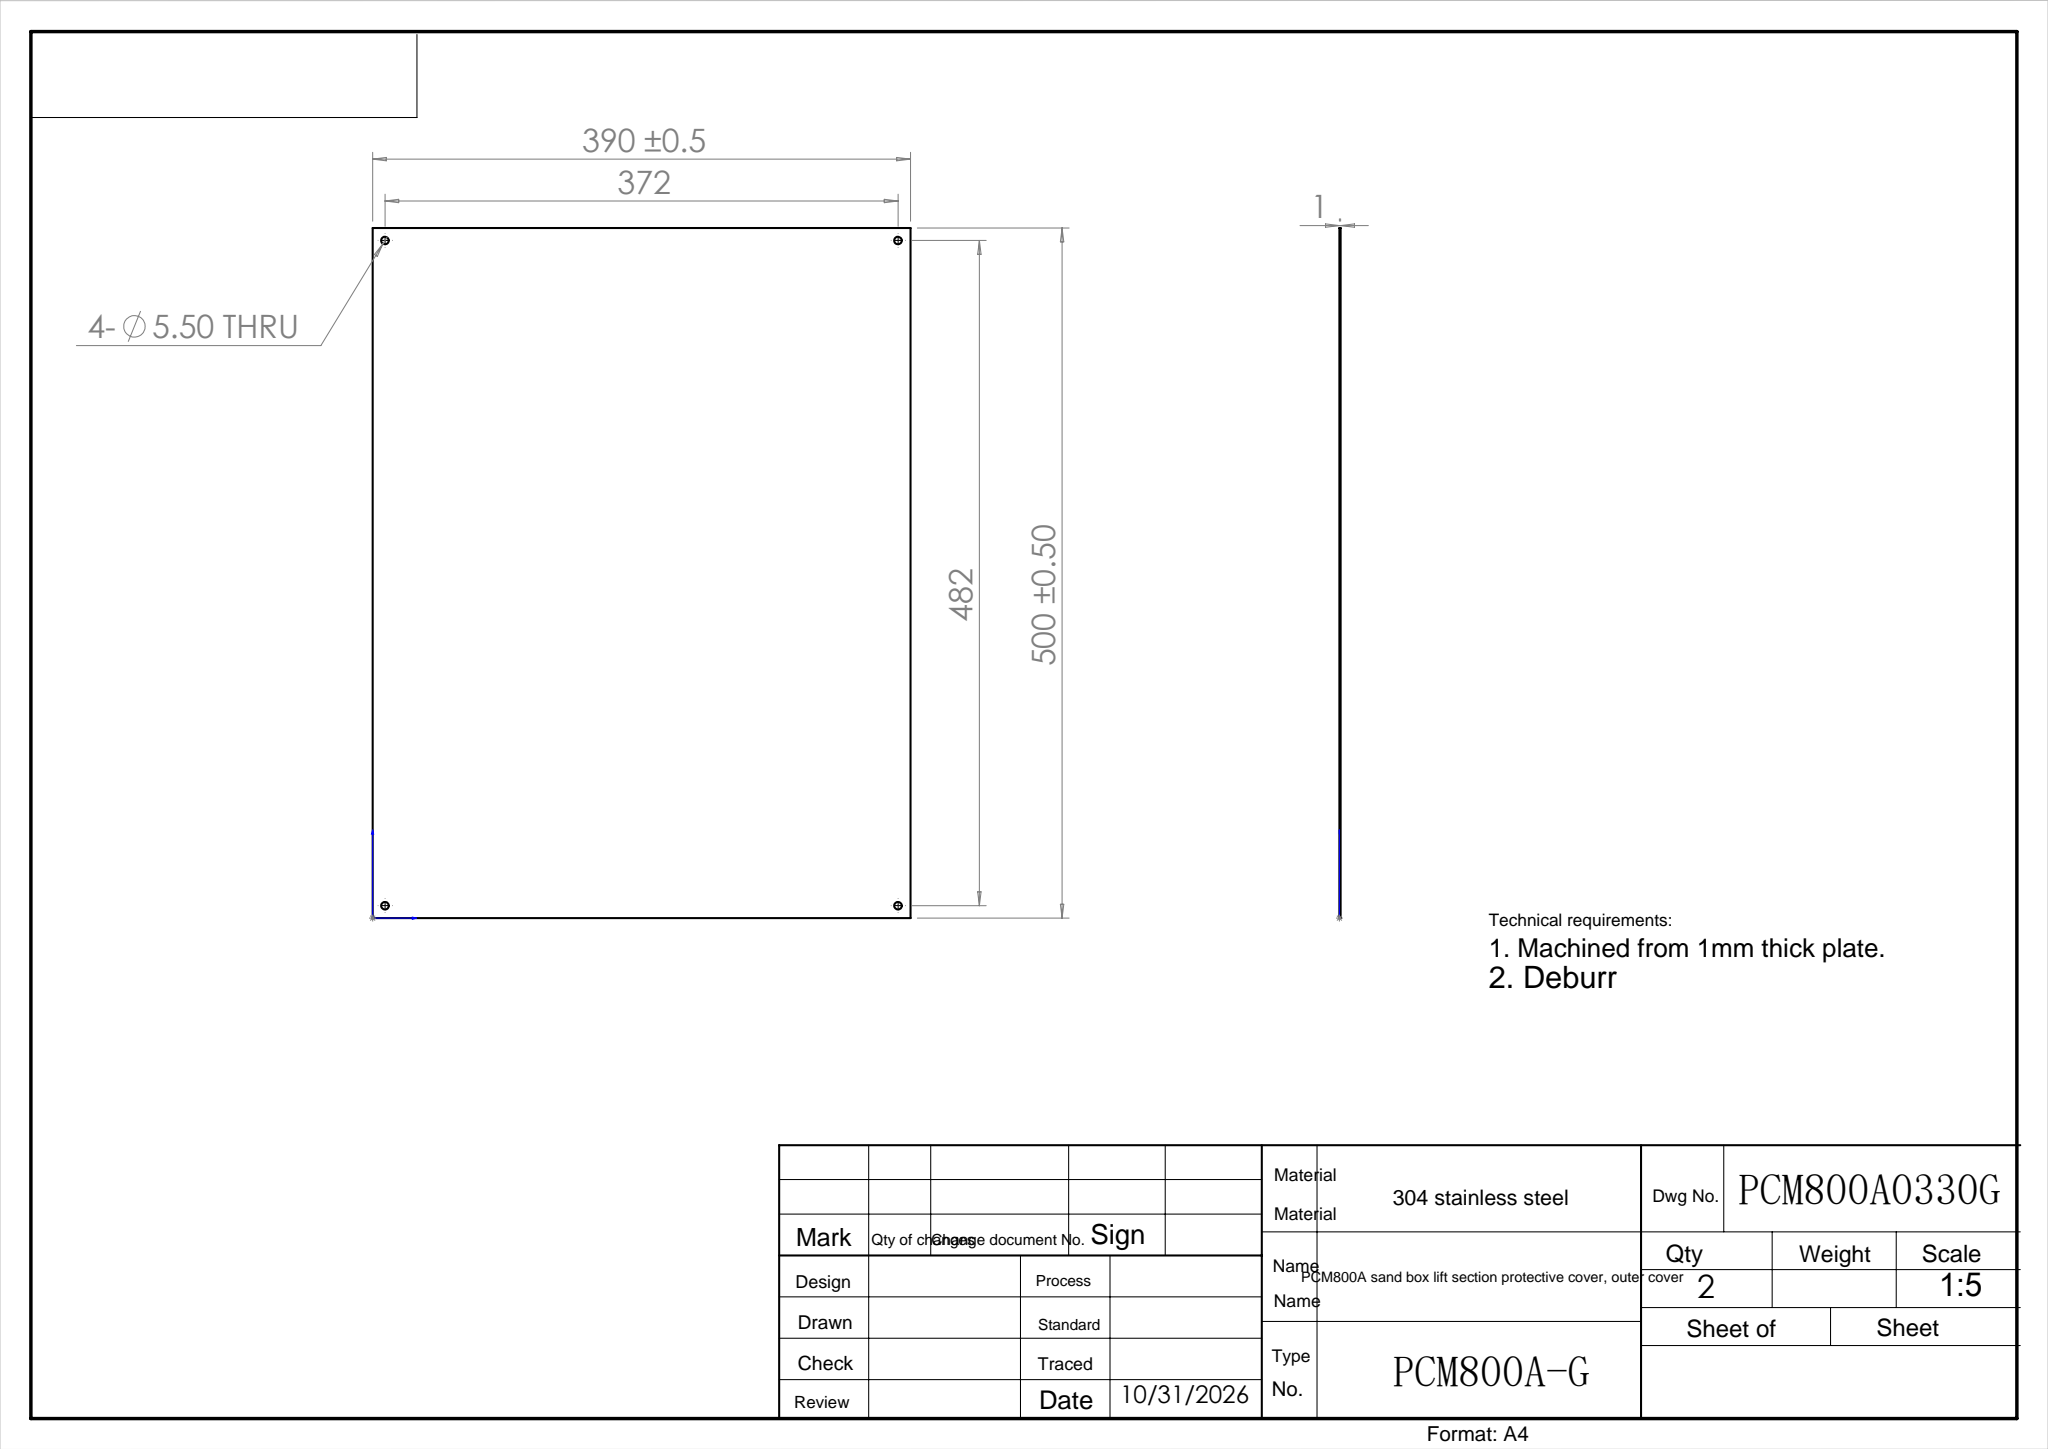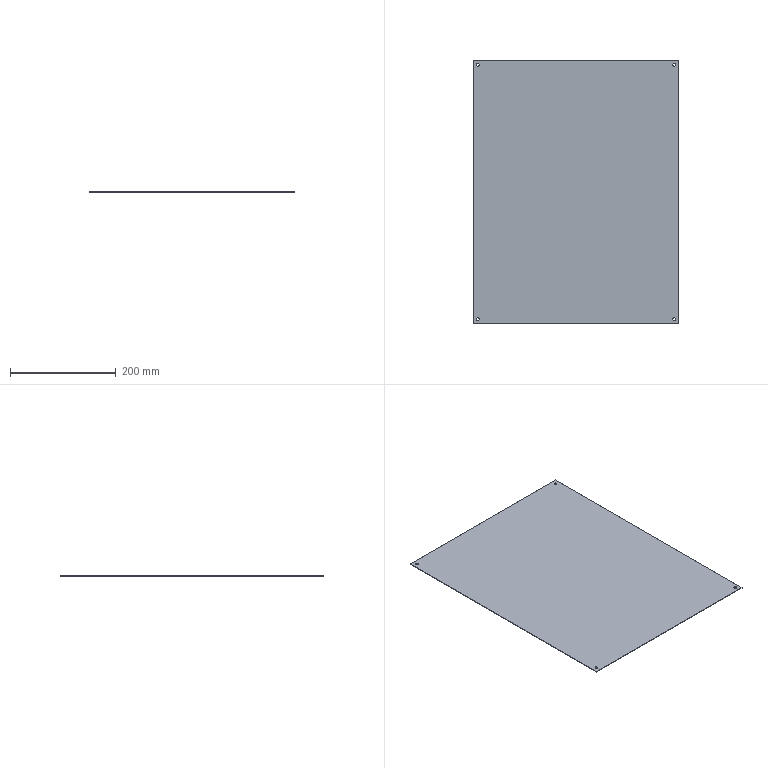Part | SolidWorks | features Extrusion 1, ICE 1 | 1 solid | 14 faces | box 390 x 500 x 1 mm | volume 194905 mm3 | cylinder 8 | plane 6 | commonest cylinder face diameters 5.5 x8
STEP:
#1=CARTESIAN_POINT('',(378.25,9.,0.));
#2=VERTEX_POINT('',#1);
#3=CARTESIAN_POINT('',(383.75,9.,0.));
#4=VERTEX_POINT('',#3);
#5=CARTESIAN_POINT('',(381.,9.,0.));
#6=DIRECTION('',(0.,0.,1.));
#7=DIRECTION('',(1.,0.,0.));
#8=AXIS2_PLACEMENT_3D('',#5,#6,#7);
#9=CIRCLE('',#8,2.75);
#10=EDGE_CURVE('',#2,#4,#9,.T.);
#11=ORIENTED_EDGE('',*,*,#10,.F.);
#12=CARTESIAN_POINT('',(378.25,9.,1.));
#13=VERTEX_POINT('',#12);
#14=CARTESIAN_POINT('',(378.25,9.,0.));
#15=DIRECTION('',(0.,0.,1.));
#16=VECTOR('',#15,1000.);
#17=LINE('',#14,#16);
#18=EDGE_CURVE('',#2,#13,#17,.T.);
#19=ORIENTED_EDGE('',*,*,#18,.T.);
#20=CARTESIAN_POINT('',(383.75,9.,1.));
#21=VERTEX_POINT('',#20);
#22=CARTESIAN_POINT('',(381.,9.,1.));
#23=DIRECTION('',(0.,0.,1.));
#24=DIRECTION('',(1.,0.,0.));
#25=AXIS2_PLACEMENT_3D('',#22,#23,#24);
#26=CIRCLE('',#25,2.75);
#27=EDGE_CURVE('',#13,#21,#26,.T.);
#28=ORIENTED_EDGE('',*,*,#27,.T.);
#29=CARTESIAN_POINT('',(383.75,9.,0.));
#30=DIRECTION('',(0.,0.,1.));
#31=VECTOR('',#30,1000.);
#32=LINE('',#29,#31);
#33=EDGE_CURVE('',#4,#21,#32,.T.);
#34=ORIENTED_EDGE('',*,*,#33,.F.);
#35=EDGE_LOOP('',(#11,#19,#28,#34));
#36=FACE_OUTER_BOUND('',#35,.T.);
#37=CARTESIAN_POINT('',(381.,9.,0.));
#38=DIRECTION('',(0.,0.,1.));
#39=DIRECTION('',(1.,0.,0.));
#40=AXIS2_PLACEMENT_3D('',#37,#38,#39);
#41=CYLINDRICAL_SURFACE('',#40,2.75);
#42=ADVANCED_FACE('',(#36),#41,.F.);
#43=CARTESIAN_POINT('',(6.25,9.,0.));
#44=VERTEX_POINT('',#43);
#45=CARTESIAN_POINT('',(11.75,9.,0.));
#46=VERTEX_POINT('',#45);
#47=CARTESIAN_POINT('',(9.,9.,0.));
#48=DIRECTION('',(0.,0.,1.));
#49=DIRECTION('',(1.,0.,0.));
#50=AXIS2_PLACEMENT_3D('',#47,#48,#49);
#51=CIRCLE('',#50,2.75);
#52=EDGE_CURVE('',#44,#46,#51,.T.);
#53=ORIENTED_EDGE('',*,*,#52,.F.);
#54=CARTESIAN_POINT('',(6.25,9.,1.));
#55=VERTEX_POINT('',#54);
#56=CARTESIAN_POINT('',(6.25,9.,0.));
#57=DIRECTION('',(0.,0.,1.));
#58=VECTOR('',#57,1000.);
#59=LINE('',#56,#58);
#60=EDGE_CURVE('',#44,#55,#59,.T.);
#61=ORIENTED_EDGE('',*,*,#60,.T.);
#62=CARTESIAN_POINT('',(11.75,9.,1.));
#63=VERTEX_POINT('',#62);
#64=CARTESIAN_POINT('',(9.,9.,1.));
#65=DIRECTION('',(0.,0.,1.));
#66=DIRECTION('',(1.,0.,0.));
#67=AXIS2_PLACEMENT_3D('',#64,#65,#66);
#68=CIRCLE('',#67,2.75);
#69=EDGE_CURVE('',#55,#63,#68,.T.);
#70=ORIENTED_EDGE('',*,*,#69,.T.);
#71=CARTESIAN_POINT('',(11.75,9.,0.));
#72=DIRECTION('',(0.,0.,1.));
#73=VECTOR('',#72,1000.);
#74=LINE('',#71,#73);
#75=EDGE_CURVE('',#46,#63,#74,.T.);
#76=ORIENTED_EDGE('',*,*,#75,.F.);
#77=EDGE_LOOP('',(#53,#61,#70,#76));
#78=FACE_OUTER_BOUND('',#77,.T.);
#79=CARTESIAN_POINT('',(9.,9.,0.));
#80=DIRECTION('',(0.,0.,1.));
#81=DIRECTION('',(1.,0.,0.));
#82=AXIS2_PLACEMENT_3D('',#79,#80,#81);
#83=CYLINDRICAL_SURFACE('',#82,2.75);
#84=ADVANCED_FACE('',(#78),#83,.F.);
#85=CARTESIAN_POINT('',(378.25,491.,0.));
#86=VERTEX_POINT('',#85);
#87=CARTESIAN_POINT('',(383.75,491.,0.));
#88=VERTEX_POINT('',#87);
#89=CARTESIAN_POINT('',(381.,491.,0.));
#90=DIRECTION('',(0.,0.,1.));
#91=DIRECTION('',(1.,0.,0.));
#92=AXIS2_PLACEMENT_3D('',#89,#90,#91);
#93=CIRCLE('',#92,2.75);
#94=EDGE_CURVE('',#86,#88,#93,.T.);
#95=ORIENTED_EDGE('',*,*,#94,.F.);
#96=CARTESIAN_POINT('',(378.25,491.,1.));
#97=VERTEX_POINT('',#96);
#98=CARTESIAN_POINT('',(378.25,491.,0.));
#99=DIRECTION('',(0.,0.,1.));
#100=VECTOR('',#99,1000.);
#101=LINE('',#98,#100);
#102=EDGE_CURVE('',#86,#97,#101,.T.);
#103=ORIENTED_EDGE('',*,*,#102,.T.);
#104=CARTESIAN_POINT('',(383.75,491.,1.));
#105=VERTEX_POINT('',#104);
#106=CARTESIAN_POINT('',(381.,491.,1.));
#107=DIRECTION('',(0.,0.,1.));
#108=DIRECTION('',(1.,0.,0.));
#109=AXIS2_PLACEMENT_3D('',#106,#107,#108);
#110=CIRCLE('',#109,2.75);
#111=EDGE_CURVE('',#97,#105,#110,.T.);
#112=ORIENTED_EDGE('',*,*,#111,.T.);
#113=CARTESIAN_POINT('',(383.75,491.,0.));
#114=DIRECTION('',(0.,0.,1.));
#115=VECTOR('',#114,1000.);
#116=LINE('',#113,#115);
#117=EDGE_CURVE('',#88,#105,#116,.T.);
#118=ORIENTED_EDGE('',*,*,#117,.F.);
#119=EDGE_LOOP('',(#95,#103,#112,#118));
#120=FACE_OUTER_BOUND('',#119,.T.);
#121=CARTESIAN_POINT('',(381.,491.,0.));
#122=DIRECTION('',(0.,0.,1.));
#123=DIRECTION('',(1.,0.,0.));
#124=AXIS2_PLACEMENT_3D('',#121,#122,#123);
#125=CYLINDRICAL_SURFACE('',#124,2.75);
#126=ADVANCED_FACE('',(#120),#125,.F.);
#127=CARTESIAN_POINT('',(6.25,491.,0.));
#128=VERTEX_POINT('',#127);
#129=CARTESIAN_POINT('',(11.75,491.,0.));
#130=VERTEX_POINT('',#129);
#131=CARTESIAN_POINT('',(9.,491.,0.));
#132=DIRECTION('',(0.,0.,1.));
#133=DIRECTION('',(1.,0.,0.));
#134=AXIS2_PLACEMENT_3D('',#131,#132,#133);
#135=CIRCLE('',#134,2.75);
#136=EDGE_CURVE('',#128,#130,#135,.T.);
#137=ORIENTED_EDGE('',*,*,#136,.F.);
#138=CARTESIAN_POINT('',(6.25,491.,1.));
#139=VERTEX_POINT('',#138);
#140=CARTESIAN_POINT('',(6.25,491.,0.));
#141=DIRECTION('',(0.,0.,1.));
#142=VECTOR('',#141,1000.);
#143=LINE('',#140,#142);
#144=EDGE_CURVE('',#128,#139,#143,.T.);
#145=ORIENTED_EDGE('',*,*,#144,.T.);
#146=CARTESIAN_POINT('',(11.75,491.,1.));
#147=VERTEX_POINT('',#146);
#148=CARTESIAN_POINT('',(9.,491.,1.));
#149=DIRECTION('',(0.,0.,1.));
#150=DIRECTION('',(1.,0.,0.));
#151=AXIS2_PLACEMENT_3D('',#148,#149,#150);
#152=CIRCLE('',#151,2.75);
#153=EDGE_CURVE('',#139,#147,#152,.T.);
#154=ORIENTED_EDGE('',*,*,#153,.T.);
#155=CARTESIAN_POINT('',(11.75,491.,0.));
#156=DIRECTION('',(0.,0.,1.));
#157=VECTOR('',#156,1000.);
#158=LINE('',#155,#157);
#159=EDGE_CURVE('',#130,#147,#158,.T.);
#160=ORIENTED_EDGE('',*,*,#159,.F.);
#161=EDGE_LOOP('',(#137,#145,#154,#160));
#162=FACE_OUTER_BOUND('',#161,.T.);
#163=CARTESIAN_POINT('',(9.,491.,0.));
#164=DIRECTION('',(0.,0.,1.));
#165=DIRECTION('',(1.,0.,0.));
#166=AXIS2_PLACEMENT_3D('',#163,#164,#165);
#167=CYLINDRICAL_SURFACE('',#166,2.75);
#168=ADVANCED_FACE('',(#162),#167,.F.);
#169=CARTESIAN_POINT('',(0.,500.,0.));
#170=VERTEX_POINT('',#169);
#171=CARTESIAN_POINT('',(0.,0.,0.));
#172=VERTEX_POINT('',#171);
#173=CARTESIAN_POINT('',(0.,0.,0.));
#174=DIRECTION('',(0.,-1.,0.));
#175=VECTOR('',#174,1000.);
#176=LINE('',#173,#175);
#177=EDGE_CURVE('',#170,#172,#176,.T.);
#178=ORIENTED_EDGE('',*,*,#177,.T.);
#179=CARTESIAN_POINT('',(0.,0.,1.));
#180=VERTEX_POINT('',#179);
#181=CARTESIAN_POINT('',(0.,0.,1.));
#182=DIRECTION('',(0.,0.,-1.));
#183=VECTOR('',#182,1000.);
#184=LINE('',#181,#183);
#185=EDGE_CURVE('',#180,#172,#184,.T.);
#186=ORIENTED_EDGE('',*,*,#185,.F.);
#187=CARTESIAN_POINT('',(0.,500.,1.));
#188=VERTEX_POINT('',#187);
#189=CARTESIAN_POINT('',(0.,0.,1.));
#190=DIRECTION('',(0.,-1.,0.));
#191=VECTOR('',#190,1000.);
#192=LINE('',#189,#191);
#193=EDGE_CURVE('',#188,#180,#192,.T.);
#194=ORIENTED_EDGE('',*,*,#193,.F.);
#195=CARTESIAN_POINT('',(0.,500.,1.));
#196=DIRECTION('',(0.,0.,-1.));
#197=VECTOR('',#196,1000.);
#198=LINE('',#195,#197);
#199=EDGE_CURVE('',#188,#170,#198,.T.);
#200=ORIENTED_EDGE('',*,*,#199,.T.);
#201=EDGE_LOOP('',(#178,#186,#194,#200));
#202=FACE_OUTER_BOUND('',#201,.T.);
#203=CARTESIAN_POINT('',(0.,0.,1.));
#204=DIRECTION('',(1.,0.,0.));
#205=DIRECTION('',(0.,0.,-1.));
#206=AXIS2_PLACEMENT_3D('',#203,#204,#205);
#207=PLANE('',#206);
#208=ADVANCED_FACE('',(#202),#207,.F.);
#209=CARTESIAN_POINT('',(390.,0.,0.));
#210=VERTEX_POINT('',#209);
#211=CARTESIAN_POINT('',(0.,0.,0.));
#212=DIRECTION('',(1.,0.,0.));
#213=VECTOR('',#212,1000.);
#214=LINE('',#211,#213);
#215=EDGE_CURVE('',#172,#210,#214,.T.);
#216=ORIENTED_EDGE('',*,*,#215,.T.);
#217=CARTESIAN_POINT('',(390.,0.,1.));
#218=VERTEX_POINT('',#217);
#219=CARTESIAN_POINT('',(390.,0.,1.));
#220=DIRECTION('',(0.,0.,-1.));
#221=VECTOR('',#220,1000.);
#222=LINE('',#219,#221);
#223=EDGE_CURVE('',#218,#210,#222,.T.);
#224=ORIENTED_EDGE('',*,*,#223,.F.);
#225=CARTESIAN_POINT('',(0.,0.,1.));
#226=DIRECTION('',(1.,0.,0.));
#227=VECTOR('',#226,1000.);
#228=LINE('',#225,#227);
#229=EDGE_CURVE('',#180,#218,#228,.T.);
#230=ORIENTED_EDGE('',*,*,#229,.F.);
#231=ORIENTED_EDGE('',*,*,#185,.T.);
#232=EDGE_LOOP('',(#216,#224,#230,#231));
#233=FACE_OUTER_BOUND('',#232,.T.);
#234=CARTESIAN_POINT('',(0.,0.,1.));
#235=DIRECTION('',(0.,1.,0.));
#236=DIRECTION('',(0.,0.,1.));
#237=AXIS2_PLACEMENT_3D('',#234,#235,#236);
#238=PLANE('',#237);
#239=ADVANCED_FACE('',(#233),#238,.F.);
#240=CARTESIAN_POINT('',(390.,500.,0.));
#241=VERTEX_POINT('',#240);
#242=CARTESIAN_POINT('',(390.,0.,0.));
#243=DIRECTION('',(0.,1.,0.));
#244=VECTOR('',#243,1000.);
#245=LINE('',#242,#244);
#246=EDGE_CURVE('',#210,#241,#245,.T.);
#247=ORIENTED_EDGE('',*,*,#246,.T.);
#248=CARTESIAN_POINT('',(390.,500.,1.));
#249=VERTEX_POINT('',#248);
#250=CARTESIAN_POINT('',(390.,500.,1.));
#251=DIRECTION('',(0.,0.,-1.));
#252=VECTOR('',#251,1000.);
#253=LINE('',#250,#252);
#254=EDGE_CURVE('',#249,#241,#253,.T.);
#255=ORIENTED_EDGE('',*,*,#254,.F.);
#256=CARTESIAN_POINT('',(390.,0.,1.));
#257=DIRECTION('',(0.,1.,0.));
#258=VECTOR('',#257,1000.);
#259=LINE('',#256,#258);
#260=EDGE_CURVE('',#218,#249,#259,.T.);
#261=ORIENTED_EDGE('',*,*,#260,.F.);
#262=ORIENTED_EDGE('',*,*,#223,.T.);
#263=EDGE_LOOP('',(#247,#255,#261,#262));
#264=FACE_OUTER_BOUND('',#263,.T.);
#265=CARTESIAN_POINT('',(390.,0.,1.));
#266=DIRECTION('',(-1.,0.,0.));
#267=DIRECTION('',(0.,0.,1.));
#268=AXIS2_PLACEMENT_3D('',#265,#266,#267);
#269=PLANE('',#268);
#270=ADVANCED_FACE('',(#264),#269,.F.);
#271=CARTESIAN_POINT('',(0.,500.,0.));
#272=DIRECTION('',(-1.,0.,0.));
#273=VECTOR('',#272,1000.);
#274=LINE('',#271,#273);
#275=EDGE_CURVE('',#241,#170,#274,.T.);
#276=ORIENTED_EDGE('',*,*,#275,.T.);
#277=ORIENTED_EDGE('',*,*,#199,.F.);
#278=CARTESIAN_POINT('',(0.,500.,1.));
#279=DIRECTION('',(-1.,0.,0.));
#280=VECTOR('',#279,1000.);
#281=LINE('',#278,#280);
#282=EDGE_CURVE('',#249,#188,#281,.T.);
#283=ORIENTED_EDGE('',*,*,#282,.F.);
#284=ORIENTED_EDGE('',*,*,#254,.T.);
#285=EDGE_LOOP('',(#276,#277,#283,#284));
#286=FACE_OUTER_BOUND('',#285,.T.);
#287=CARTESIAN_POINT('',(0.,500.,1.));
#288=DIRECTION('',(0.,-1.,0.));
#289=DIRECTION('',(0.,0.,-1.));
#290=AXIS2_PLACEMENT_3D('',#287,#288,#289);
#291=PLANE('',#290);
#292=ADVANCED_FACE('',(#286),#291,.F.);
#293=CARTESIAN_POINT('',(381.,9.,1.));
#294=DIRECTION('',(0.,0.,1.));
#295=DIRECTION('',(1.,0.,0.));
#296=AXIS2_PLACEMENT_3D('',#293,#294,#295);
#297=CIRCLE('',#296,2.75);
#298=EDGE_CURVE('',#21,#13,#297,.T.);
#299=ORIENTED_EDGE('',*,*,#298,.F.);
#300=ORIENTED_EDGE('',*,*,#27,.F.);
#301=EDGE_LOOP('',(#299,#300));
#302=FACE_BOUND('',#301,.T.);
#303=CARTESIAN_POINT('',(9.,9.,1.));
#304=DIRECTION('',(0.,0.,1.));
#305=DIRECTION('',(1.,0.,0.));
#306=AXIS2_PLACEMENT_3D('',#303,#304,#305);
#307=CIRCLE('',#306,2.75);
#308=EDGE_CURVE('',#63,#55,#307,.T.);
#309=ORIENTED_EDGE('',*,*,#308,.F.);
#310=ORIENTED_EDGE('',*,*,#69,.F.);
#311=EDGE_LOOP('',(#309,#310));
#312=FACE_BOUND('',#311,.T.);
#313=CARTESIAN_POINT('',(381.,491.,1.));
#314=DIRECTION('',(0.,0.,1.));
#315=DIRECTION('',(1.,0.,0.));
#316=AXIS2_PLACEMENT_3D('',#313,#314,#315);
#317=CIRCLE('',#316,2.75);
#318=EDGE_CURVE('',#105,#97,#317,.T.);
#319=ORIENTED_EDGE('',*,*,#318,.F.);
#320=ORIENTED_EDGE('',*,*,#111,.F.);
#321=EDGE_LOOP('',(#319,#320));
#322=FACE_BOUND('',#321,.T.);
#323=CARTESIAN_POINT('',(9.,491.,1.));
#324=DIRECTION('',(0.,0.,1.));
#325=DIRECTION('',(1.,0.,0.));
#326=AXIS2_PLACEMENT_3D('',#323,#324,#325);
#327=CIRCLE('',#326,2.75);
#328=EDGE_CURVE('',#147,#139,#327,.T.);
#329=ORIENTED_EDGE('',*,*,#328,.F.);
#330=ORIENTED_EDGE('',*,*,#153,.F.);
#331=EDGE_LOOP('',(#329,#330));
#332=FACE_BOUND('',#331,.T.);
#333=ORIENTED_EDGE('',*,*,#193,.T.);
#334=ORIENTED_EDGE('',*,*,#229,.T.);
#335=ORIENTED_EDGE('',*,*,#260,.T.);
#336=ORIENTED_EDGE('',*,*,#282,.T.);
#337=EDGE_LOOP('',(#333,#334,#335,#336));
#338=FACE_OUTER_BOUND('',#337,.T.);
#339=CARTESIAN_POINT('',(0.,500.,1.));
#340=DIRECTION('',(0.,0.,-1.));
#341=DIRECTION('',(-1.,0.,0.));
#342=AXIS2_PLACEMENT_3D('',#339,#340,#341);
#343=PLANE('',#342);
#344=ADVANCED_FACE('',(#302,#312,#322,#332,#338),#343,.F.);
#345=CARTESIAN_POINT('',(381.,9.,0.));
#346=DIRECTION('',(0.,0.,1.));
#347=DIRECTION('',(1.,0.,0.));
#348=AXIS2_PLACEMENT_3D('',#345,#346,#347);
#349=CIRCLE('',#348,2.75);
#350=EDGE_CURVE('',#4,#2,#349,.T.);
#351=ORIENTED_EDGE('',*,*,#350,.T.);
#352=ORIENTED_EDGE('',*,*,#10,.T.);
#353=EDGE_LOOP('',(#351,#352));
#354=FACE_BOUND('',#353,.T.);
#355=CARTESIAN_POINT('',(9.,9.,0.));
#356=DIRECTION('',(0.,0.,1.));
#357=DIRECTION('',(1.,0.,0.));
#358=AXIS2_PLACEMENT_3D('',#355,#356,#357);
#359=CIRCLE('',#358,2.75);
#360=EDGE_CURVE('',#46,#44,#359,.T.);
#361=ORIENTED_EDGE('',*,*,#360,.T.);
#362=ORIENTED_EDGE('',*,*,#52,.T.);
#363=EDGE_LOOP('',(#361,#362));
#364=FACE_BOUND('',#363,.T.);
#365=CARTESIAN_POINT('',(381.,491.,0.));
#366=DIRECTION('',(0.,0.,1.));
#367=DIRECTION('',(1.,0.,0.));
#368=AXIS2_PLACEMENT_3D('',#365,#366,#367);
#369=CIRCLE('',#368,2.75);
#370=EDGE_CURVE('',#88,#86,#369,.T.);
#371=ORIENTED_EDGE('',*,*,#370,.T.);
#372=ORIENTED_EDGE('',*,*,#94,.T.);
#373=EDGE_LOOP('',(#371,#372));
#374=FACE_BOUND('',#373,.T.);
#375=CARTESIAN_POINT('',(9.,491.,0.));
#376=DIRECTION('',(0.,0.,1.));
#377=DIRECTION('',(1.,0.,0.));
#378=AXIS2_PLACEMENT_3D('',#375,#376,#377);
#379=CIRCLE('',#378,2.75);
#380=EDGE_CURVE('',#130,#128,#379,.T.);
#381=ORIENTED_EDGE('',*,*,#380,.T.);
#382=ORIENTED_EDGE('',*,*,#136,.T.);
#383=EDGE_LOOP('',(#381,#382));
#384=FACE_BOUND('',#383,.T.);
#385=ORIENTED_EDGE('',*,*,#177,.F.);
#386=ORIENTED_EDGE('',*,*,#275,.F.);
#387=ORIENTED_EDGE('',*,*,#246,.F.);
#388=ORIENTED_EDGE('',*,*,#215,.F.);
#389=EDGE_LOOP('',(#385,#386,#387,#388));
#390=FACE_OUTER_BOUND('',#389,.T.);
#391=CARTESIAN_POINT('',(0.,500.,0.));
#392=DIRECTION('',(0.,0.,-1.));
#393=DIRECTION('',(-1.,0.,0.));
#394=AXIS2_PLACEMENT_3D('',#391,#392,#393);
#395=PLANE('',#394);
#396=ADVANCED_FACE('',(#354,#364,#374,#384,#390),#395,.T.);
#397=ORIENTED_EDGE('',*,*,#144,.F.);
#398=ORIENTED_EDGE('',*,*,#380,.F.);
#399=ORIENTED_EDGE('',*,*,#159,.T.);
#400=ORIENTED_EDGE('',*,*,#328,.T.);
#401=EDGE_LOOP('',(#397,#398,#399,#400));
#402=FACE_OUTER_BOUND('',#401,.T.);
#403=CARTESIAN_POINT('',(9.,491.,0.));
#404=DIRECTION('',(0.,0.,1.));
#405=DIRECTION('',(1.,0.,0.));
#406=AXIS2_PLACEMENT_3D('',#403,#404,#405);
#407=CYLINDRICAL_SURFACE('',#406,2.75);
#408=ADVANCED_FACE('',(#402),#407,.F.);
#409=ORIENTED_EDGE('',*,*,#102,.F.);
#410=ORIENTED_EDGE('',*,*,#370,.F.);
#411=ORIENTED_EDGE('',*,*,#117,.T.);
#412=ORIENTED_EDGE('',*,*,#318,.T.);
#413=EDGE_LOOP('',(#409,#410,#411,#412));
#414=FACE_OUTER_BOUND('',#413,.T.);
#415=CARTESIAN_POINT('',(381.,491.,0.));
#416=DIRECTION('',(0.,0.,1.));
#417=DIRECTION('',(1.,0.,0.));
#418=AXIS2_PLACEMENT_3D('',#415,#416,#417);
#419=CYLINDRICAL_SURFACE('',#418,2.75);
#420=ADVANCED_FACE('',(#414),#419,.F.);
#421=ORIENTED_EDGE('',*,*,#60,.F.);
#422=ORIENTED_EDGE('',*,*,#360,.F.);
#423=ORIENTED_EDGE('',*,*,#75,.T.);
#424=ORIENTED_EDGE('',*,*,#308,.T.);
#425=EDGE_LOOP('',(#421,#422,#423,#424));
#426=FACE_OUTER_BOUND('',#425,.T.);
#427=CARTESIAN_POINT('',(9.,9.,0.));
#428=DIRECTION('',(0.,0.,1.));
#429=DIRECTION('',(1.,0.,0.));
#430=AXIS2_PLACEMENT_3D('',#427,#428,#429);
#431=CYLINDRICAL_SURFACE('',#430,2.75);
#432=ADVANCED_FACE('',(#426),#431,.F.);
#433=ORIENTED_EDGE('',*,*,#18,.F.);
#434=ORIENTED_EDGE('',*,*,#350,.F.);
#435=ORIENTED_EDGE('',*,*,#33,.T.);
#436=ORIENTED_EDGE('',*,*,#298,.T.);
#437=EDGE_LOOP('',(#433,#434,#435,#436));
#438=FACE_OUTER_BOUND('',#437,.T.);
#439=CARTESIAN_POINT('',(381.,9.,0.));
#440=DIRECTION('',(0.,0.,1.));
#441=DIRECTION('',(1.,0.,0.));
#442=AXIS2_PLACEMENT_3D('',#439,#440,#441);
#443=CYLINDRICAL_SURFACE('',#442,2.75);
#444=ADVANCED_FACE('',(#438),#443,.F.);
#445=CLOSED_SHELL('',(#42,#84,#126,#168,#208,#239,#270,#292,#344,#396,#408,#420,#432,#444));
#446=MANIFOLD_SOLID_BREP('',#445);
#447=CARTESIAN_POINT('',(0.,0.,0.));
#448=DIRECTION('',(0.,0.,1.));
#449=DIRECTION('',(1.,0.,0.));
#450=AXIS2_PLACEMENT_3D('',#447,#448,#449);
#451=(LENGTH_UNIT()NAMED_UNIT(*)SI_UNIT(.MILLI.,.METRE.));
#452=UNCERTAINTY_MEASURE_WITH_UNIT(LENGTH_MEASURE(0.00001),#451,'','');
#453=(NAMED_UNIT(*)PLANE_ANGLE_UNIT()SI_UNIT($,.RADIAN.));
#454=(NAMED_UNIT(*)SI_UNIT($,.STERADIAN.)SOLID_ANGLE_UNIT());
#455=(GEOMETRIC_REPRESENTATION_CONTEXT(3)GLOBAL_UNCERTAINTY_ASSIGNED_CONTEXT((#452))GLOBAL_UNIT_ASSIGNED_CONTEXT((#451,#453,#454))REPRESENTATION_CONTEXT('',''));
#456=ADVANCED_BREP_SHAPE_REPRESENTATION('',(#446,#450),#455);